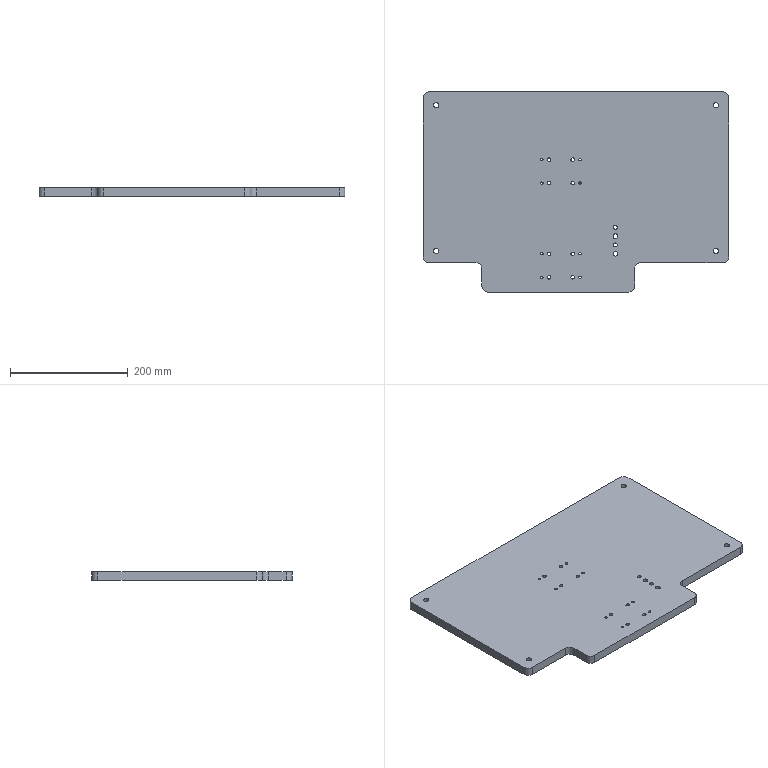Part | STEP file | SN10_008_001_PLACA | 1 solid | 42 faces | box 520 x 340 x 15 mm | volume 2444343 mm3 | cylinder 32 | plane 10 | commonest cylinder face diameters 4.134 x8 6 x8 20 x8 9 x4 6.647 x2 8 x2